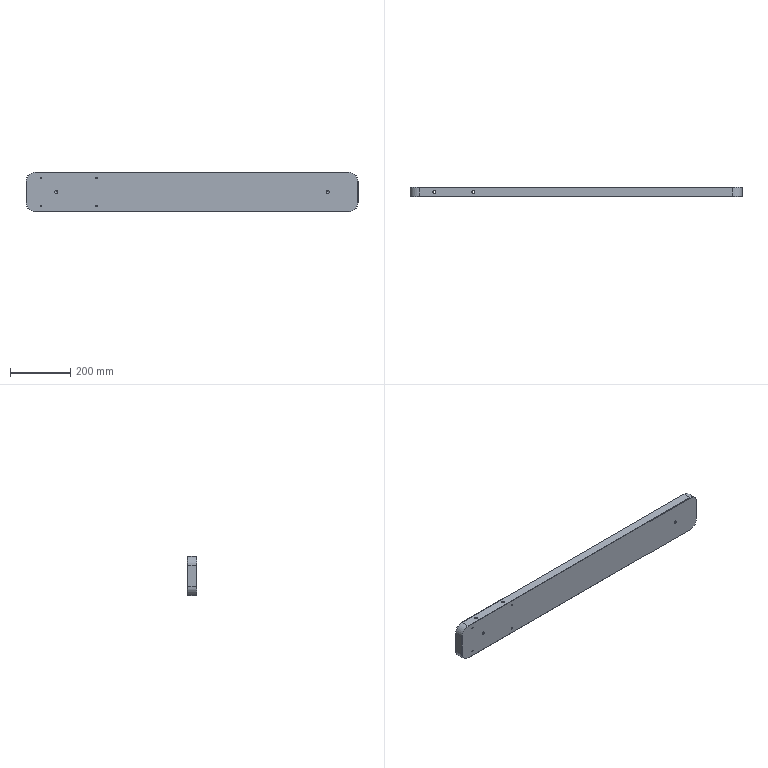Part | SolidWorks | features HoleWzd 3, Chamfer 1, Extrusion 1, Fillet 1 | 1 solid | 50 faces | box 1100 x 30 x 130 mm | volume 4243037 mm3 | cylinder 20 | cone 16 | plane 14 | commonest cylinder face diameters 5 x8 8.5 x4 10.2 x4 60 x4
STEP:
#1=CARTESIAN_POINT('',(-474.25,15.,64.225));
#2=VERTEX_POINT('',#1);
#3=CARTESIAN_POINT('',(-465.75,15.,64.225));
#4=VERTEX_POINT('',#3);
#5=CARTESIAN_POINT('',(-470.,15.,64.225));
#6=DIRECTION('',(0.,0.,1.));
#7=DIRECTION('',(1.,0.,0.));
#8=AXIS2_PLACEMENT_3D('',#5,#6,#7);
#9=CIRCLE('',#8,4.25);
#10=EDGE_CURVE('',#2,#4,#9,.T.);
#11=ORIENTED_EDGE('',*,*,#10,.F.);
#12=CARTESIAN_POINT('',(-475.025,15.,65.));
#13=VERTEX_POINT('',#12);
#14=CARTESIAN_POINT('',(-475.025,15.,65.));
#15=DIRECTION('',(-0.7071,0.,0.7071));
#16=VECTOR('',#15,1000.);
#17=LINE('',#14,#16);
#18=EDGE_CURVE('',#2,#13,#17,.T.);
#19=ORIENTED_EDGE('',*,*,#18,.T.);
#20=CARTESIAN_POINT('',(-464.975,15.,65.));
#21=VERTEX_POINT('',#20);
#22=CARTESIAN_POINT('',(-470.,15.,65.));
#23=DIRECTION('',(0.,0.,1.));
#24=DIRECTION('',(1.,0.,0.));
#25=AXIS2_PLACEMENT_3D('',#22,#23,#24);
#26=CIRCLE('',#25,5.025);
#27=EDGE_CURVE('',#13,#21,#26,.T.);
#28=ORIENTED_EDGE('',*,*,#27,.T.);
#29=CARTESIAN_POINT('',(-464.975,15.,65.));
#30=DIRECTION('',(0.7071,0.,0.7071));
#31=VECTOR('',#30,1000.);
#32=LINE('',#29,#31);
#33=EDGE_CURVE('',#4,#21,#32,.T.);
#34=ORIENTED_EDGE('',*,*,#33,.F.);
#35=EDGE_LOOP('',(#11,#19,#28,#34));
#36=FACE_OUTER_BOUND('',#35,.T.);
#37=CARTESIAN_POINT('',(-470.,15.,65.));
#38=DIRECTION('',(0.,0.,1.));
#39=DIRECTION('',(1.,0.,0.));
#40=AXIS2_PLACEMENT_3D('',#37,#38,#39);
#41=CONICAL_SURFACE('',#40,5.025,0.7854);
#42=ADVANCED_FACE('',(#36),#41,.F.);
#43=CARTESIAN_POINT('',(-474.25,15.,-65.));
#44=VERTEX_POINT('',#43);
#45=CARTESIAN_POINT('',(-465.75,15.,-65.));
#46=VERTEX_POINT('',#45);
#47=CARTESIAN_POINT('',(-470.,15.,-65.));
#48=DIRECTION('',(0.,0.,1.));
#49=DIRECTION('',(1.,0.,0.));
#50=AXIS2_PLACEMENT_3D('',#47,#48,#49);
#51=CIRCLE('',#50,4.25);
#52=EDGE_CURVE('',#44,#46,#51,.T.);
#53=ORIENTED_EDGE('',*,*,#52,.F.);
#54=CARTESIAN_POINT('',(-474.25,15.,65.));
#55=DIRECTION('',(0.,0.,1.));
#56=VECTOR('',#55,1000.);
#57=LINE('',#54,#56);
#58=EDGE_CURVE('',#44,#2,#57,.T.);
#59=ORIENTED_EDGE('',*,*,#58,.T.);
#60=ORIENTED_EDGE('',*,*,#10,.T.);
#61=CARTESIAN_POINT('',(-465.75,15.,65.));
#62=DIRECTION('',(0.,0.,1.));
#63=VECTOR('',#62,1000.);
#64=LINE('',#61,#63);
#65=EDGE_CURVE('',#46,#4,#64,.T.);
#66=ORIENTED_EDGE('',*,*,#65,.F.);
#67=EDGE_LOOP('',(#53,#59,#60,#66));
#68=FACE_OUTER_BOUND('',#67,.T.);
#69=CARTESIAN_POINT('',(-470.,15.,65.));
#70=DIRECTION('',(0.,0.,1.));
#71=DIRECTION('',(1.,0.,0.));
#72=AXIS2_PLACEMENT_3D('',#69,#70,#71);
#73=CYLINDRICAL_SURFACE('',#72,4.25);
#74=ADVANCED_FACE('',(#68),#73,.F.);
#75=CARTESIAN_POINT('',(-344.25,15.,64.225));
#76=VERTEX_POINT('',#75);
#77=CARTESIAN_POINT('',(-335.75,15.,64.225));
#78=VERTEX_POINT('',#77);
#79=CARTESIAN_POINT('',(-340.,15.,64.225));
#80=DIRECTION('',(0.,0.,1.));
#81=DIRECTION('',(1.,0.,0.));
#82=AXIS2_PLACEMENT_3D('',#79,#80,#81);
#83=CIRCLE('',#82,4.25);
#84=EDGE_CURVE('',#76,#78,#83,.T.);
#85=ORIENTED_EDGE('',*,*,#84,.F.);
#86=CARTESIAN_POINT('',(-345.025,15.,65.));
#87=VERTEX_POINT('',#86);
#88=CARTESIAN_POINT('',(-345.025,15.,65.));
#89=DIRECTION('',(-0.7071,0.,0.7071));
#90=VECTOR('',#89,1000.);
#91=LINE('',#88,#90);
#92=EDGE_CURVE('',#76,#87,#91,.T.);
#93=ORIENTED_EDGE('',*,*,#92,.T.);
#94=CARTESIAN_POINT('',(-334.975,15.,65.));
#95=VERTEX_POINT('',#94);
#96=CARTESIAN_POINT('',(-340.,15.,65.));
#97=DIRECTION('',(0.,0.,1.));
#98=DIRECTION('',(1.,0.,0.));
#99=AXIS2_PLACEMENT_3D('',#96,#97,#98);
#100=CIRCLE('',#99,5.025);
#101=EDGE_CURVE('',#87,#95,#100,.T.);
#102=ORIENTED_EDGE('',*,*,#101,.T.);
#103=CARTESIAN_POINT('',(-334.975,15.,65.));
#104=DIRECTION('',(0.7071,0.,0.7071));
#105=VECTOR('',#104,1000.);
#106=LINE('',#103,#105);
#107=EDGE_CURVE('',#78,#95,#106,.T.);
#108=ORIENTED_EDGE('',*,*,#107,.F.);
#109=EDGE_LOOP('',(#85,#93,#102,#108));
#110=FACE_OUTER_BOUND('',#109,.T.);
#111=CARTESIAN_POINT('',(-340.,15.,65.));
#112=DIRECTION('',(0.,0.,1.));
#113=DIRECTION('',(1.,0.,0.));
#114=AXIS2_PLACEMENT_3D('',#111,#112,#113);
#115=CONICAL_SURFACE('',#114,5.025,0.7854);
#116=ADVANCED_FACE('',(#110),#115,.F.);
#117=CARTESIAN_POINT('',(-344.25,15.,-65.));
#118=VERTEX_POINT('',#117);
#119=CARTESIAN_POINT('',(-335.75,15.,-65.));
#120=VERTEX_POINT('',#119);
#121=CARTESIAN_POINT('',(-340.,15.,-65.));
#122=DIRECTION('',(0.,0.,1.));
#123=DIRECTION('',(1.,0.,0.));
#124=AXIS2_PLACEMENT_3D('',#121,#122,#123);
#125=CIRCLE('',#124,4.25);
#126=EDGE_CURVE('',#118,#120,#125,.T.);
#127=ORIENTED_EDGE('',*,*,#126,.F.);
#128=CARTESIAN_POINT('',(-344.25,15.,65.));
#129=DIRECTION('',(0.,0.,1.));
#130=VECTOR('',#129,1000.);
#131=LINE('',#128,#130);
#132=EDGE_CURVE('',#118,#76,#131,.T.);
#133=ORIENTED_EDGE('',*,*,#132,.T.);
#134=ORIENTED_EDGE('',*,*,#84,.T.);
#135=CARTESIAN_POINT('',(-335.75,15.,65.));
#136=DIRECTION('',(0.,0.,1.));
#137=VECTOR('',#136,1000.);
#138=LINE('',#135,#137);
#139=EDGE_CURVE('',#120,#78,#138,.T.);
#140=ORIENTED_EDGE('',*,*,#139,.F.);
#141=EDGE_LOOP('',(#127,#133,#134,#140));
#142=FACE_OUTER_BOUND('',#141,.T.);
#143=CARTESIAN_POINT('',(-340.,15.,65.));
#144=DIRECTION('',(0.,0.,1.));
#145=DIRECTION('',(1.,0.,0.));
#146=AXIS2_PLACEMENT_3D('',#143,#144,#145);
#147=CYLINDRICAL_SURFACE('',#146,4.25);
#148=ADVANCED_FACE('',(#142),#147,.F.);
#149=CARTESIAN_POINT('',(450.,25.,5.1));
#150=VERTEX_POINT('',#149);
#151=CARTESIAN_POINT('',(450.,25.,-5.1));
#152=VERTEX_POINT('',#151);
#153=CARTESIAN_POINT('',(450.,25.,0.));
#154=DIRECTION('',(0.,-1.,0.));
#155=DIRECTION('',(0.,0.,-1.));
#156=AXIS2_PLACEMENT_3D('',#153,#154,#155);
#157=CIRCLE('',#156,5.1);
#158=EDGE_CURVE('',#150,#152,#157,.T.);
#159=ORIENTED_EDGE('',*,*,#158,.F.);
#160=CARTESIAN_POINT('',(450.,0.,5.1));
#161=VERTEX_POINT('',#160);
#162=CARTESIAN_POINT('',(450.,0.,5.1));
#163=DIRECTION('',(0.,-1.,0.));
#164=VECTOR('',#163,1000.);
#165=LINE('',#162,#164);
#166=EDGE_CURVE('',#150,#161,#165,.T.);
#167=ORIENTED_EDGE('',*,*,#166,.T.);
#168=CARTESIAN_POINT('',(450.,0.,-5.1));
#169=VERTEX_POINT('',#168);
#170=CARTESIAN_POINT('',(450.,0.,0.));
#171=DIRECTION('',(0.,-1.,0.));
#172=DIRECTION('',(0.,0.,-1.));
#173=AXIS2_PLACEMENT_3D('',#170,#171,#172);
#174=CIRCLE('',#173,5.1);
#175=EDGE_CURVE('',#161,#169,#174,.T.);
#176=ORIENTED_EDGE('',*,*,#175,.T.);
#177=CARTESIAN_POINT('',(450.,0.,-5.1));
#178=DIRECTION('',(0.,-1.,0.));
#179=VECTOR('',#178,1000.);
#180=LINE('',#177,#179);
#181=EDGE_CURVE('',#152,#169,#180,.T.);
#182=ORIENTED_EDGE('',*,*,#181,.F.);
#183=EDGE_LOOP('',(#159,#167,#176,#182));
#184=FACE_OUTER_BOUND('',#183,.T.);
#185=CARTESIAN_POINT('',(450.,0.,0.));
#186=DIRECTION('',(0.,-1.,0.));
#187=DIRECTION('',(0.,0.,-1.));
#188=AXIS2_PLACEMENT_3D('',#185,#186,#187);
#189=CYLINDRICAL_SURFACE('',#188,5.1);
#190=ADVANCED_FACE('',(#184),#189,.F.);
#191=CARTESIAN_POINT('',(450.,28.064,0.));
#192=VERTEX_POINT('',#191);
#193=CARTESIAN_POINT('',(450.,25.,-5.1));
#194=DIRECTION('',(0.,-0.515,-0.8572));
#195=VECTOR('',#194,1000.);
#196=LINE('',#193,#195);
#197=EDGE_CURVE('',#192,#152,#196,.T.);
#198=ORIENTED_EDGE('',*,*,#197,.F.);
#199=CARTESIAN_POINT('',(450.,25.,5.1));
#200=DIRECTION('',(0.,-0.515,0.8572));
#201=VECTOR('',#200,1000.);
#202=LINE('',#199,#201);
#203=EDGE_CURVE('',#192,#150,#202,.T.);
#204=ORIENTED_EDGE('',*,*,#203,.T.);
#205=ORIENTED_EDGE('',*,*,#158,.T.);
#206=EDGE_LOOP('',(#198,#204,#205));
#207=FACE_OUTER_BOUND('',#206,.T.);
#208=CARTESIAN_POINT('',(450.,25.,0.));
#209=DIRECTION('',(0.,-1.,0.));
#210=DIRECTION('',(0.,0.,-1.));
#211=AXIS2_PLACEMENT_3D('',#208,#209,#210);
#212=CONICAL_SURFACE('',#211,5.1,1.03);
#213=ADVANCED_FACE('',(#207),#212,.F.);
#214=CARTESIAN_POINT('',(-450.,25.,5.1));
#215=VERTEX_POINT('',#214);
#216=CARTESIAN_POINT('',(-450.,25.,-5.1));
#217=VERTEX_POINT('',#216);
#218=CARTESIAN_POINT('',(-450.,25.,0.));
#219=DIRECTION('',(0.,-1.,0.));
#220=DIRECTION('',(0.,0.,-1.));
#221=AXIS2_PLACEMENT_3D('',#218,#219,#220);
#222=CIRCLE('',#221,5.1);
#223=EDGE_CURVE('',#215,#217,#222,.T.);
#224=ORIENTED_EDGE('',*,*,#223,.F.);
#225=CARTESIAN_POINT('',(-450.,0.,5.1));
#226=VERTEX_POINT('',#225);
#227=CARTESIAN_POINT('',(-450.,0.,5.1));
#228=DIRECTION('',(0.,-1.,0.));
#229=VECTOR('',#228,1000.);
#230=LINE('',#227,#229);
#231=EDGE_CURVE('',#215,#226,#230,.T.);
#232=ORIENTED_EDGE('',*,*,#231,.T.);
#233=CARTESIAN_POINT('',(-450.,0.,-5.1));
#234=VERTEX_POINT('',#233);
#235=CARTESIAN_POINT('',(-450.,0.,0.));
#236=DIRECTION('',(0.,-1.,0.));
#237=DIRECTION('',(0.,0.,-1.));
#238=AXIS2_PLACEMENT_3D('',#235,#236,#237);
#239=CIRCLE('',#238,5.1);
#240=EDGE_CURVE('',#226,#234,#239,.T.);
#241=ORIENTED_EDGE('',*,*,#240,.T.);
#242=CARTESIAN_POINT('',(-450.,0.,-5.1));
#243=DIRECTION('',(0.,-1.,0.));
#244=VECTOR('',#243,1000.);
#245=LINE('',#242,#244);
#246=EDGE_CURVE('',#217,#234,#245,.T.);
#247=ORIENTED_EDGE('',*,*,#246,.F.);
#248=EDGE_LOOP('',(#224,#232,#241,#247));
#249=FACE_OUTER_BOUND('',#248,.T.);
#250=CARTESIAN_POINT('',(-450.,0.,0.));
#251=DIRECTION('',(0.,-1.,0.));
#252=DIRECTION('',(0.,0.,-1.));
#253=AXIS2_PLACEMENT_3D('',#250,#251,#252);
#254=CYLINDRICAL_SURFACE('',#253,5.1);
#255=ADVANCED_FACE('',(#249),#254,.F.);
#256=CARTESIAN_POINT('',(-450.,28.064,0.));
#257=VERTEX_POINT('',#256);
#258=CARTESIAN_POINT('',(-450.,25.,-5.1));
#259=DIRECTION('',(0.,-0.515,-0.8572));
#260=VECTOR('',#259,1000.);
#261=LINE('',#258,#260);
#262=EDGE_CURVE('',#257,#217,#261,.T.);
#263=ORIENTED_EDGE('',*,*,#262,.F.);
#264=CARTESIAN_POINT('',(-450.,25.,5.1));
#265=DIRECTION('',(0.,-0.515,0.8572));
#266=VECTOR('',#265,1000.);
#267=LINE('',#264,#266);
#268=EDGE_CURVE('',#257,#215,#267,.T.);
#269=ORIENTED_EDGE('',*,*,#268,.T.);
#270=ORIENTED_EDGE('',*,*,#223,.T.);
#271=EDGE_LOOP('',(#263,#269,#270));
#272=FACE_OUTER_BOUND('',#271,.T.);
#273=CARTESIAN_POINT('',(-450.,25.,0.));
#274=DIRECTION('',(0.,-1.,0.));
#275=DIRECTION('',(0.,0.,-1.));
#276=AXIS2_PLACEMENT_3D('',#273,#274,#275);
#277=CONICAL_SURFACE('',#276,5.1,1.03);
#278=ADVANCED_FACE('',(#272),#277,.F.);
#279=CARTESIAN_POINT('',(-316.,0.,-49.5));
#280=VERTEX_POINT('',#279);
#281=CARTESIAN_POINT('',(-316.,0.,-44.5));
#282=VERTEX_POINT('',#281);
#283=CARTESIAN_POINT('',(-316.,0.,-47.));
#284=DIRECTION('',(0.,1.,0.));
#285=DIRECTION('',(0.,0.,1.));
#286=AXIS2_PLACEMENT_3D('',#283,#284,#285);
#287=CIRCLE('',#286,2.5);
#288=EDGE_CURVE('',#280,#282,#287,.T.);
#289=ORIENTED_EDGE('',*,*,#288,.F.);
#290=CARTESIAN_POINT('',(-316.,30.,-49.5));
#291=VERTEX_POINT('',#290);
#292=CARTESIAN_POINT('',(-316.,30.,-49.5));
#293=DIRECTION('',(0.,1.,0.));
#294=VECTOR('',#293,1000.);
#295=LINE('',#292,#294);
#296=EDGE_CURVE('',#280,#291,#295,.T.);
#297=ORIENTED_EDGE('',*,*,#296,.T.);
#298=CARTESIAN_POINT('',(-316.,30.,-44.5));
#299=VERTEX_POINT('',#298);
#300=CARTESIAN_POINT('',(-316.,30.,-47.));
#301=DIRECTION('',(0.,1.,0.));
#302=DIRECTION('',(0.,0.,1.));
#303=AXIS2_PLACEMENT_3D('',#300,#301,#302);
#304=CIRCLE('',#303,2.5);
#305=EDGE_CURVE('',#291,#299,#304,.T.);
#306=ORIENTED_EDGE('',*,*,#305,.T.);
#307=CARTESIAN_POINT('',(-316.,30.,-44.5));
#308=DIRECTION('',(0.,1.,0.));
#309=VECTOR('',#308,1000.);
#310=LINE('',#307,#309);
#311=EDGE_CURVE('',#282,#299,#310,.T.);
#312=ORIENTED_EDGE('',*,*,#311,.F.);
#313=EDGE_LOOP('',(#289,#297,#306,#312));
#314=FACE_OUTER_BOUND('',#313,.T.);
#315=CARTESIAN_POINT('',(-316.,30.,-47.));
#316=DIRECTION('',(0.,1.,0.));
#317=DIRECTION('',(0.,0.,1.));
#318=AXIS2_PLACEMENT_3D('',#315,#316,#317);
#319=CYLINDRICAL_SURFACE('',#318,2.5);
#320=ADVANCED_FACE('',(#314),#319,.F.);
#321=CARTESIAN_POINT('',(-316.,0.,44.5));
#322=VERTEX_POINT('',#321);
#323=CARTESIAN_POINT('',(-316.,0.,49.5));
#324=VERTEX_POINT('',#323);
#325=CARTESIAN_POINT('',(-316.,0.,47.));
#326=DIRECTION('',(0.,1.,0.));
#327=DIRECTION('',(0.,0.,1.));
#328=AXIS2_PLACEMENT_3D('',#325,#326,#327);
#329=CIRCLE('',#328,2.5);
#330=EDGE_CURVE('',#322,#324,#329,.T.);
#331=ORIENTED_EDGE('',*,*,#330,.F.);
#332=CARTESIAN_POINT('',(-316.,30.,44.5));
#333=VERTEX_POINT('',#332);
#334=CARTESIAN_POINT('',(-316.,30.,44.5));
#335=DIRECTION('',(0.,1.,0.));
#336=VECTOR('',#335,1000.);
#337=LINE('',#334,#336);
#338=EDGE_CURVE('',#322,#333,#337,.T.);
#339=ORIENTED_EDGE('',*,*,#338,.T.);
#340=CARTESIAN_POINT('',(-316.,30.,49.5));
#341=VERTEX_POINT('',#340);
#342=CARTESIAN_POINT('',(-316.,30.,47.));
#343=DIRECTION('',(0.,1.,0.));
#344=DIRECTION('',(0.,0.,1.));
#345=AXIS2_PLACEMENT_3D('',#342,#343,#344);
#346=CIRCLE('',#345,2.5);
#347=EDGE_CURVE('',#333,#341,#346,.T.);
#348=ORIENTED_EDGE('',*,*,#347,.T.);
#349=CARTESIAN_POINT('',(-316.,30.,49.5));
#350=DIRECTION('',(0.,1.,0.));
#351=VECTOR('',#350,1000.);
#352=LINE('',#349,#351);
#353=EDGE_CURVE('',#324,#341,#352,.T.);
#354=ORIENTED_EDGE('',*,*,#353,.F.);
#355=EDGE_LOOP('',(#331,#339,#348,#354));
#356=FACE_OUTER_BOUND('',#355,.T.);
#357=CARTESIAN_POINT('',(-316.,30.,47.));
#358=DIRECTION('',(0.,1.,0.));
#359=DIRECTION('',(0.,0.,1.));
#360=AXIS2_PLACEMENT_3D('',#357,#358,#359);
#361=CYLINDRICAL_SURFACE('',#360,2.5);
#362=ADVANCED_FACE('',(#356),#361,.F.);
#363=CARTESIAN_POINT('',(-500.,0.,-49.5));
#364=VERTEX_POINT('',#363);
#365=CARTESIAN_POINT('',(-500.,0.,-44.5));
#366=VERTEX_POINT('',#365);
#367=CARTESIAN_POINT('',(-500.,0.,-47.));
#368=DIRECTION('',(0.,1.,0.));
#369=DIRECTION('',(0.,0.,1.));
#370=AXIS2_PLACEMENT_3D('',#367,#368,#369);
#371=CIRCLE('',#370,2.5);
#372=EDGE_CURVE('',#364,#366,#371,.T.);
#373=ORIENTED_EDGE('',*,*,#372,.F.);
#374=CARTESIAN_POINT('',(-500.,30.,-49.5));
#375=VERTEX_POINT('',#374);
#376=CARTESIAN_POINT('',(-500.,30.,-49.5));
#377=DIRECTION('',(0.,1.,0.));
#378=VECTOR('',#377,1000.);
#379=LINE('',#376,#378);
#380=EDGE_CURVE('',#364,#375,#379,.T.);
#381=ORIENTED_EDGE('',*,*,#380,.T.);
#382=CARTESIAN_POINT('',(-500.,30.,-44.5));
#383=VERTEX_POINT('',#382);
#384=CARTESIAN_POINT('',(-500.,30.,-47.));
#385=DIRECTION('',(0.,1.,0.));
#386=DIRECTION('',(0.,0.,1.));
#387=AXIS2_PLACEMENT_3D('',#384,#385,#386);
#388=CIRCLE('',#387,2.5);
#389=EDGE_CURVE('',#375,#383,#388,.T.);
#390=ORIENTED_EDGE('',*,*,#389,.T.);
#391=CARTESIAN_POINT('',(-500.,30.,-44.5));
#392=DIRECTION('',(0.,1.,0.));
#393=VECTOR('',#392,1000.);
#394=LINE('',#391,#393);
#395=EDGE_CURVE('',#366,#383,#394,.T.);
#396=ORIENTED_EDGE('',*,*,#395,.F.);
#397=EDGE_LOOP('',(#373,#381,#390,#396));
#398=FACE_OUTER_BOUND('',#397,.T.);
#399=CARTESIAN_POINT('',(-500.,30.,-47.));
#400=DIRECTION('',(0.,1.,0.));
#401=DIRECTION('',(0.,0.,1.));
#402=AXIS2_PLACEMENT_3D('',#399,#400,#401);
#403=CYLINDRICAL_SURFACE('',#402,2.5);
#404=ADVANCED_FACE('',(#398),#403,.F.);
#405=CARTESIAN_POINT('',(-500.,0.,44.5));
#406=VERTEX_POINT('',#405);
#407=CARTESIAN_POINT('',(-500.,0.,49.5));
#408=VERTEX_POINT('',#407);
#409=CARTESIAN_POINT('',(-500.,0.,47.));
#410=DIRECTION('',(0.,1.,0.));
#411=DIRECTION('',(0.,0.,1.));
#412=AXIS2_PLACEMENT_3D('',#409,#410,#411);
#413=CIRCLE('',#412,2.5);
#414=EDGE_CURVE('',#406,#408,#413,.T.);
#415=ORIENTED_EDGE('',*,*,#414,.F.);
#416=CARTESIAN_POINT('',(-500.,30.,44.5));
#417=VERTEX_POINT('',#416);
#418=CARTESIAN_POINT('',(-500.,30.,44.5));
#419=DIRECTION('',(0.,1.,0.));
#420=VECTOR('',#419,1000.);
#421=LINE('',#418,#420);
#422=EDGE_CURVE('',#406,#417,#421,.T.);
#423=ORIENTED_EDGE('',*,*,#422,.T.);
#424=CARTESIAN_POINT('',(-500.,30.,49.5));
#425=VERTEX_POINT('',#424);
#426=CARTESIAN_POINT('',(-500.,30.,47.));
#427=DIRECTION('',(0.,1.,0.));
#428=DIRECTION('',(0.,0.,1.));
#429=AXIS2_PLACEMENT_3D('',#426,#427,#428);
#430=CIRCLE('',#429,2.5);
#431=EDGE_CURVE('',#417,#425,#430,.T.);
#432=ORIENTED_EDGE('',*,*,#431,.T.);
#433=CARTESIAN_POINT('',(-500.,30.,49.5));
#434=DIRECTION('',(0.,1.,0.));
#435=VECTOR('',#434,1000.);
#436=LINE('',#433,#435);
#437=EDGE_CURVE('',#408,#425,#436,.T.);
#438=ORIENTED_EDGE('',*,*,#437,.F.);
#439=EDGE_LOOP('',(#415,#423,#432,#438));
#440=FACE_OUTER_BOUND('',#439,.T.);
#441=CARTESIAN_POINT('',(-500.,30.,47.));
#442=DIRECTION('',(0.,1.,0.));
#443=DIRECTION('',(0.,0.,1.));
#444=AXIS2_PLACEMENT_3D('',#441,#442,#443);
#445=CYLINDRICAL_SURFACE('',#444,2.5);
#446=ADVANCED_FACE('',(#440),#445,.F.);
#447=CARTESIAN_POINT('',(550.,29.,35.));
#448=VERTEX_POINT('',#447);
#449=CARTESIAN_POINT('',(550.,1.,35.));
#450=VERTEX_POINT('',#449);
#451=CARTESIAN_POINT('',(550.,30.,35.));
#452=DIRECTION('',(0.,-1.,0.));
#453=VECTOR('',#452,1000.);
#454=LINE('',#451,#453);
#455=EDGE_CURVE('',#448,#450,#454,.T.);
#456=ORIENTED_EDGE('',*,*,#455,.T.);
#457=CARTESIAN_POINT('',(550.,1.,-35.));
#458=VERTEX_POINT('',#457);
#459=CARTESIAN_POINT('',(550.,1.,-35.));
#460=DIRECTION('',(0.,0.,-1.));
#461=VECTOR('',#460,1000.);
#462=LINE('',#459,#461);
#463=EDGE_CURVE('',#450,#458,#462,.T.);
#464=ORIENTED_EDGE('',*,*,#463,.T.);
#465=CARTESIAN_POINT('',(550.,29.,-35.));
#466=VERTEX_POINT('',#465);
#467=CARTESIAN_POINT('',(550.,30.,-35.));
#468=DIRECTION('',(0.,1.,0.));
#469=VECTOR('',#468,1000.);
#470=LINE('',#467,#469);
#471=EDGE_CURVE('',#458,#466,#470,.T.);
#472=ORIENTED_EDGE('',*,*,#471,.T.);
#473=CARTESIAN_POINT('',(550.,29.,65.));
#474=DIRECTION('',(0.,0.,1.));
#475=VECTOR('',#474,1000.);
#476=LINE('',#473,#475);
#477=EDGE_CURVE('',#466,#448,#476,.T.);
#478=ORIENTED_EDGE('',*,*,#477,.T.);
#479=EDGE_LOOP('',(#456,#464,#472,#478));
#480=FACE_OUTER_BOUND('',#479,.T.);
#481=CARTESIAN_POINT('',(550.,30.,65.));
#482=DIRECTION('',(-1.,0.,0.));
#483=DIRECTION('',(0.,0.,1.));
#484=AXIS2_PLACEMENT_3D('',#481,#482,#483);
#485=PLANE('',#484);
#486=ADVANCED_FACE('',(#480),#485,.F.);
#487=CARTESIAN_POINT('',(-470.,15.,-65.));
#488=DIRECTION('',(0.,0.,1.));
#489=DIRECTION('',(1.,0.,0.));
#490=AXIS2_PLACEMENT_3D('',#487,#488,#489);
#491=CIRCLE('',#490,4.25);
#492=EDGE_CURVE('',#46,#44,#491,.T.);
#493=ORIENTED_EDGE('',*,*,#492,.T.);
#494=ORIENTED_EDGE('',*,*,#52,.T.);
#495=EDGE_LOOP('',(#493,#494));
#496=FACE_BOUND('',#495,.T.);
#497=CARTESIAN_POINT('',(-340.,15.,-65.));
#498=DIRECTION('',(0.,0.,1.));
#499=DIRECTION('',(1.,0.,0.));
#500=AXIS2_PLACEMENT_3D('',#497,#498,#499);
#501=CIRCLE('',#500,4.25);
#502=EDGE_CURVE('',#120,#118,#501,.T.);
#503=ORIENTED_EDGE('',*,*,#502,.T.);
#504=ORIENTED_EDGE('',*,*,#126,.T.);
#505=EDGE_LOOP('',(#503,#504));
#506=FACE_BOUND('',#505,.T.);
#507=CARTESIAN_POINT('',(520.,29.,-65.));
#508=VERTEX_POINT('',#507);
#509=CARTESIAN_POINT('',(520.,1.,-65.));
#510=VERTEX_POINT('',#509);
#511=CARTESIAN_POINT('',(520.,30.,-65.));
#512=DIRECTION('',(0.,-1.,0.));
#513=VECTOR('',#512,1000.);
#514=LINE('',#511,#513);
#515=EDGE_CURVE('',#508,#510,#514,.T.);
#516=ORIENTED_EDGE('',*,*,#515,.T.);
#517=CARTESIAN_POINT('',(-520.,1.,-65.));
#518=VERTEX_POINT('',#517);
#519=CARTESIAN_POINT('',(-520.,1.,-65.));
#520=DIRECTION('',(-1.,0.,0.));
#521=VECTOR('',#520,1000.);
#522=LINE('',#519,#521);
#523=EDGE_CURVE('',#510,#518,#522,.T.);
#524=ORIENTED_EDGE('',*,*,#523,.T.);
#525=CARTESIAN_POINT('',(-520.,29.,-65.));
#526=VERTEX_POINT('',#525);
#527=CARTESIAN_POINT('',(-520.,30.,-65.));
#528=DIRECTION('',(0.,1.,0.));
#529=VECTOR('',#528,1000.);
#530=LINE('',#527,#529);
#531=EDGE_CURVE('',#518,#526,#530,.T.);
#532=ORIENTED_EDGE('',*,*,#531,.T.);
#533=CARTESIAN_POINT('',(-550.,29.,-65.));
#534=DIRECTION('',(1.,0.,0.));
#535=VECTOR('',#534,1000.);
#536=LINE('',#533,#535);
#537=EDGE_CURVE('',#526,#508,#536,.T.);
#538=ORIENTED_EDGE('',*,*,#537,.T.);
#539=EDGE_LOOP('',(#516,#524,#532,#538));
#540=FACE_OUTER_BOUND('',#539,.T.);
#541=CARTESIAN_POINT('',(-550.,30.,-65.));
#542=DIRECTION('',(0.,0.,1.));
#543=DIRECTION('',(1.,0.,0.));
#544=AXIS2_PLACEMENT_3D('',#541,#542,#543);
#545=PLANE('',#544);
#546=ADVANCED_FACE('',(#496,#506,#540),#545,.F.);
#547=CARTESIAN_POINT('',(-550.,29.,-35.));
#548=VERTEX_POINT('',#547);
#549=CARTESIAN_POINT('',(-550.,1.,-35.));
#550=VERTEX_POINT('',#549);
#551=CARTESIAN_POINT('',(-550.,30.,-35.));
#552=DIRECTION('',(0.,-1.,0.));
#553=VECTOR('',#552,1000.);
#554=LINE('',#551,#553);
#555=EDGE_CURVE('',#548,#550,#554,.T.);
#556=ORIENTED_EDGE('',*,*,#555,.T.);
#557=CARTESIAN_POINT('',(-550.,1.,35.));
#558=VERTEX_POINT('',#557);
#559=CARTESIAN_POINT('',(-550.,1.,35.));
#560=DIRECTION('',(0.,0.,1.));
#561=VECTOR('',#560,1000.);
#562=LINE('',#559,#561);
#563=EDGE_CURVE('',#550,#558,#562,.T.);
#564=ORIENTED_EDGE('',*,*,#563,.T.);
#565=CARTESIAN_POINT('',(-550.,29.,35.));
#566=VERTEX_POINT('',#565);
#567=CARTESIAN_POINT('',(-550.,30.,35.));
#568=DIRECTION('',(0.,1.,0.));
#569=VECTOR('',#568,1000.);
#570=LINE('',#567,#569);
#571=EDGE_CURVE('',#558,#566,#570,.T.);
#572=ORIENTED_EDGE('',*,*,#571,.T.);
#573=CARTESIAN_POINT('',(-550.,29.,65.));
#574=DIRECTION('',(0.,0.,-1.));
#575=VECTOR('',#574,1000.);
#576=LINE('',#573,#575);
#577=EDGE_CURVE('',#566,#548,#576,.T.);
#578=ORIENTED_EDGE('',*,*,#577,.T.);
#579=EDGE_LOOP('',(#556,#564,#572,#578));
#580=FACE_OUTER_BOUND('',#579,.T.);
#581=CARTESIAN_POINT('',(-550.,30.,65.));
#582=DIRECTION('',(1.,0.,0.));
#583=DIRECTION('',(0.,0.,-1.));
#584=AXIS2_PLACEMENT_3D('',#581,#582,#583);
#585=PLANE('',#584);
#586=ADVANCED_FACE('',(#580),#585,.F.);
#587=CARTESIAN_POINT('',(-470.,15.,65.));
#588=DIRECTION('',(0.,0.,1.));
#589=DIRECTION('',(1.,0.,0.));
#590=AXIS2_PLACEMENT_3D('',#587,#588,#589);
#591=CIRCLE('',#590,5.025);
#592=EDGE_CURVE('',#21,#13,#591,.T.);
#593=ORIENTED_EDGE('',*,*,#592,.F.);
#594=ORIENTED_EDGE('',*,*,#27,.F.);
#595=EDGE_LOOP('',(#593,#594));
#596=FACE_BOUND('',#595,.T.);
#597=CARTESIAN_POINT('',(-340.,15.,65.));
#598=DIRECTION('',(0.,0.,1.));
#599=DIRECTION('',(1.,0.,0.));
#600=AXIS2_PLACEMENT_3D('',#597,#598,#599);
#601=CIRCLE('',#600,5.025);
#602=EDGE_CURVE('',#95,#87,#601,.T.);
#603=ORIENTED_EDGE('',*,*,#602,.F.);
#604=ORIENTED_EDGE('',*,*,#101,.F.);
#605=EDGE_LOOP('',(#603,#604));
#606=FACE_BOUND('',#605,.T.);
#607=CARTESIAN_POINT('',(-520.,29.,65.));
#608=VERTEX_POINT('',#607);
#609=CARTESIAN_POINT('',(-520.,1.,65.));
#610=VERTEX_POINT('',#609);
#611=CARTESIAN_POINT('',(-520.,30.,65.));
#612=DIRECTION('',(0.,-1.,0.));
#613=VECTOR('',#612,1000.);
#614=LINE('',#611,#613);
#615=EDGE_CURVE('',#608,#610,#614,.T.);
#616=ORIENTED_EDGE('',*,*,#615,.T.);
#617=CARTESIAN_POINT('',(520.,1.,65.));
#618=VERTEX_POINT('',#617);
#619=CARTESIAN_POINT('',(520.,1.,65.));
#620=DIRECTION('',(1.,0.,0.));
#621=VECTOR('',#620,1000.);
#622=LINE('',#619,#621);
#623=EDGE_CURVE('',#610,#618,#622,.T.);
#624=ORIENTED_EDGE('',*,*,#623,.T.);
#625=CARTESIAN_POINT('',(520.,29.,65.));
#626=VERTEX_POINT('',#625);
#627=CARTESIAN_POINT('',(520.,30.,65.));
#628=DIRECTION('',(0.,1.,0.));
#629=VECTOR('',#628,1000.);
#630=LINE('',#627,#629);
#631=EDGE_CURVE('',#618,#626,#630,.T.);
#632=ORIENTED_EDGE('',*,*,#631,.T.);
#633=CARTESIAN_POINT('',(-550.,29.,65.));
#634=DIRECTION('',(-1.,0.,0.));
#635=VECTOR('',#634,1000.);
#636=LINE('',#633,#635);
#637=EDGE_CURVE('',#626,#608,#636,.T.);
#638=ORIENTED_EDGE('',*,*,#637,.T.);
#639=EDGE_LOOP('',(#616,#624,#632,#638));
#640=FACE_OUTER_BOUND('',#639,.T.);
#641=CARTESIAN_POINT('',(-550.,30.,65.));
#642=DIRECTION('',(0.,0.,-1.));
#643=DIRECTION('',(-1.,0.,0.));
#644=AXIS2_PLACEMENT_3D('',#641,#642,#643);
#645=PLANE('',#644);
#646=ADVANCED_FACE('',(#596,#606,#640),#645,.F.);
#647=CARTESIAN_POINT('',(520.,30.,64.));
#648=VERTEX_POINT('',#647);
#649=CARTESIAN_POINT('',(549.,30.,35.));
#650=VERTEX_POINT('',#649);
#651=CARTESIAN_POINT('',(520.,30.,35.));
#652=DIRECTION('',(0.,1.,0.));
#653=DIRECTION('',(0.,0.,-1.));
#654=AXIS2_PLACEMENT_3D('',#651,#652,#653);
#655=CIRCLE('',#654,29.);
#656=EDGE_CURVE('',#648,#650,#655,.T.);
#657=ORIENTED_EDGE('',*,*,#656,.T.);
#658=CARTESIAN_POINT('',(549.,30.,-35.));
#659=VERTEX_POINT('',#658);
#660=CARTESIAN_POINT('',(549.,30.,0.));
#661=DIRECTION('',(0.,0.,-1.));
#662=VECTOR('',#661,1000.);
#663=LINE('',#660,#662);
#664=EDGE_CURVE('',#650,#659,#663,.T.);
#665=ORIENTED_EDGE('',*,*,#664,.T.);
#666=CARTESIAN_POINT('',(520.,30.,-64.));
#667=VERTEX_POINT('',#666);
#668=CARTESIAN_POINT('',(520.,30.,-35.));
#669=DIRECTION('',(0.,1.,0.));
#670=DIRECTION('',(0.,0.,-1.));
#671=AXIS2_PLACEMENT_3D('',#668,#669,#670);
#672=CIRCLE('',#671,29.);
#673=EDGE_CURVE('',#659,#667,#672,.T.);
#674=ORIENTED_EDGE('',*,*,#673,.T.);
#675=CARTESIAN_POINT('',(-520.,30.,-64.));
#676=VERTEX_POINT('',#675);
#677=CARTESIAN_POINT('',(0.,30.,-64.));
#678=DIRECTION('',(-1.,0.,0.));
#679=VECTOR('',#678,1000.);
#680=LINE('',#677,#679);
#681=EDGE_CURVE('',#667,#676,#680,.T.);
#682=ORIENTED_EDGE('',*,*,#681,.T.);
#683=CARTESIAN_POINT('',(-549.,30.,-35.));
#684=VERTEX_POINT('',#683);
#685=CARTESIAN_POINT('',(-520.,30.,-35.));
#686=DIRECTION('',(0.,1.,0.));
#687=DIRECTION('',(0.,0.,-1.));
#688=AXIS2_PLACEMENT_3D('',#685,#686,#687);
#689=CIRCLE('',#688,29.);
#690=EDGE_CURVE('',#676,#684,#689,.T.);
#691=ORIENTED_EDGE('',*,*,#690,.T.);
#692=CARTESIAN_POINT('',(-549.,30.,35.));
#693=VERTEX_POINT('',#692);
#694=CARTESIAN_POINT('',(-549.,30.,0.));
#695=DIRECTION('',(0.,0.,1.));
#696=VECTOR('',#695,1000.);
#697=LINE('',#694,#696);
#698=EDGE_CURVE('',#684,#693,#697,.T.);
#699=ORIENTED_EDGE('',*,*,#698,.T.);
#700=CARTESIAN_POINT('',(-520.,30.,64.));
#701=VERTEX_POINT('',#700);
#702=CARTESIAN_POINT('',(-520.,30.,35.));
#703=DIRECTION('',(0.,1.,0.));
#704=DIRECTION('',(0.,0.,-1.));
#705=AXIS2_PLACEMENT_3D('',#702,#703,#704);
#706=CIRCLE('',#705,29.);
#707=EDGE_CURVE('',#693,#701,#706,.T.);
#708=ORIENTED_EDGE('',*,*,#707,.T.);
#709=CARTESIAN_POINT('',(0.,30.,64.));
#710=DIRECTION('',(1.,0.,0.));
#711=VECTOR('',#710,1000.);
#712=LINE('',#709,#711);
#713=EDGE_CURVE('',#701,#648,#712,.T.);
#714=ORIENTED_EDGE('',*,*,#713,.T.);
#715=EDGE_LOOP('',(#657,#665,#674,#682,#691,#699,#708,#714));
#716=FACE_OUTER_BOUND('',#715,.T.);
#717=CARTESIAN_POINT('',(-316.,30.,-47.));
#718=DIRECTION('',(0.,1.,0.));
#719=DIRECTION('',(0.,0.,1.));
#720=AXIS2_PLACEMENT_3D('',#717,#718,#719);
#721=CIRCLE('',#720,2.5);
#722=EDGE_CURVE('',#299,#291,#721,.T.);
#723=ORIENTED_EDGE('',*,*,#722,.F.);
#724=ORIENTED_EDGE('',*,*,#305,.F.);
#725=EDGE_LOOP('',(#723,#724));
#726=FACE_BOUND('',#725,.T.);
#727=CARTESIAN_POINT('',(-316.,30.,47.));
#728=DIRECTION('',(0.,1.,0.));
#729=DIRECTION('',(0.,0.,1.));
#730=AXIS2_PLACEMENT_3D('',#727,#728,#729);
#731=CIRCLE('',#730,2.5);
#732=EDGE_CURVE('',#341,#333,#731,.T.);
#733=ORIENTED_EDGE('',*,*,#732,.F.);
#734=ORIENTED_EDGE('',*,*,#347,.F.);
#735=EDGE_LOOP('',(#733,#734));
#736=FACE_BOUND('',#735,.T.);
#737=CARTESIAN_POINT('',(-500.,30.,-47.));
#738=DIRECTION('',(0.,1.,0.));
#739=DIRECTION('',(0.,0.,1.));
#740=AXIS2_PLACEMENT_3D('',#737,#738,#739);
#741=CIRCLE('',#740,2.5);
#742=EDGE_CURVE('',#383,#375,#741,.T.);
#743=ORIENTED_EDGE('',*,*,#742,.F.);
#744=ORIENTED_EDGE('',*,*,#389,.F.);
#745=EDGE_LOOP('',(#743,#744));
#746=FACE_BOUND('',#745,.T.);
#747=CARTESIAN_POINT('',(-500.,30.,47.));
#748=DIRECTION('',(0.,1.,0.));
#749=DIRECTION('',(0.,0.,1.));
#750=AXIS2_PLACEMENT_3D('',#747,#748,#749);
#751=CIRCLE('',#750,2.5);
#752=EDGE_CURVE('',#425,#417,#751,.T.);
#753=ORIENTED_EDGE('',*,*,#752,.F.);
#754=ORIENTED_EDGE('',*,*,#431,.F.);
#755=EDGE_LOOP('',(#753,#754));
#756=FACE_BOUND('',#755,.T.);
#757=CARTESIAN_POINT('',(0.,30.,0.));
#758=DIRECTION('',(0.,-1.,0.));
#759=DIRECTION('',(0.,0.,-1.));
#760=AXIS2_PLACEMENT_3D('',#757,#758,#759);
#761=PLANE('',#760);
#762=ADVANCED_FACE('',(#716,#726,#736,#746,#756),#761,.F.);
#763=CARTESIAN_POINT('',(549.,0.,35.));
#764=VERTEX_POINT('',#763);
#765=CARTESIAN_POINT('',(520.,0.,64.));
#766=VERTEX_POINT('',#765);
#767=CARTESIAN_POINT('',(520.,0.,35.));
#768=DIRECTION('',(0.,-1.,0.));
#769=DIRECTION('',(0.,0.,-1.));
#770=AXIS2_PLACEMENT_3D('',#767,#768,#769);
#771=CIRCLE('',#770,29.);
#772=EDGE_CURVE('',#764,#766,#771,.T.);
#773=ORIENTED_EDGE('',*,*,#772,.T.);
#774=CARTESIAN_POINT('',(-520.,0.,64.));
#775=VERTEX_POINT('',#774);
#776=CARTESIAN_POINT('',(-520.,0.,64.));
#777=DIRECTION('',(-1.,0.,0.));
#778=VECTOR('',#777,1000.);
#779=LINE('',#776,#778);
#780=EDGE_CURVE('',#766,#775,#779,.T.);
#781=ORIENTED_EDGE('',*,*,#780,.T.);
#782=CARTESIAN_POINT('',(-549.,0.,35.));
#783=VERTEX_POINT('',#782);
#784=CARTESIAN_POINT('',(-520.,0.,35.));
#785=DIRECTION('',(0.,-1.,0.));
#786=DIRECTION('',(0.,0.,-1.));
#787=AXIS2_PLACEMENT_3D('',#784,#785,#786);
#788=CIRCLE('',#787,29.);
#789=EDGE_CURVE('',#775,#783,#788,.T.);
#790=ORIENTED_EDGE('',*,*,#789,.T.);
#791=CARTESIAN_POINT('',(-549.,0.,-35.));
#792=VERTEX_POINT('',#791);
#793=CARTESIAN_POINT('',(-549.,0.,-35.));
#794=DIRECTION('',(0.,0.,-1.));
#795=VECTOR('',#794,1000.);
#796=LINE('',#793,#795);
#797=EDGE_CURVE('',#783,#792,#796,.T.);
#798=ORIENTED_EDGE('',*,*,#797,.T.);
#799=CARTESIAN_POINT('',(-520.,0.,-64.));
#800=VERTEX_POINT('',#799);
#801=CARTESIAN_POINT('',(-520.,0.,-35.));
#802=DIRECTION('',(0.,-1.,0.));
#803=DIRECTION('',(0.,0.,-1.));
#804=AXIS2_PLACEMENT_3D('',#801,#802,#803);
#805=CIRCLE('',#804,29.);
#806=EDGE_CURVE('',#792,#800,#805,.T.);
#807=ORIENTED_EDGE('',*,*,#806,.T.);
#808=CARTESIAN_POINT('',(520.,0.,-64.));
#809=VERTEX_POINT('',#808);
#810=CARTESIAN_POINT('',(520.,0.,-64.));
#811=DIRECTION('',(1.,0.,0.));
#812=VECTOR('',#811,1000.);
#813=LINE('',#810,#812);
#814=EDGE_CURVE('',#800,#809,#813,.T.);
#815=ORIENTED_EDGE('',*,*,#814,.T.);
#816=CARTESIAN_POINT('',(549.,0.,-35.));
#817=VERTEX_POINT('',#816);
#818=CARTESIAN_POINT('',(520.,0.,-35.));
#819=DIRECTION('',(0.,-1.,0.));
#820=DIRECTION('',(0.,0.,-1.));
#821=AXIS2_PLACEMENT_3D('',#818,#819,#820);
#822=CIRCLE('',#821,29.);
#823=EDGE_CURVE('',#809,#817,#822,.T.);
#824=ORIENTED_EDGE('',*,*,#823,.T.);
#825=CARTESIAN_POINT('',(549.,0.,35.));
#826=DIRECTION('',(0.,0.,1.));
#827=VECTOR('',#826,1000.);
#828=LINE('',#825,#827);
#829=EDGE_CURVE('',#817,#764,#828,.T.);
#830=ORIENTED_EDGE('',*,*,#829,.T.);
#831=EDGE_LOOP('',(#773,#781,#790,#798,#807,#815,#824,#830));
#832=FACE_OUTER_BOUND('',#831,.T.);
#833=CARTESIAN_POINT('',(450.,0.,0.));
#834=DIRECTION('',(0.,-1.,0.));
#835=DIRECTION('',(0.,0.,-1.));
#836=AXIS2_PLACEMENT_3D('',#833,#834,#835);
#837=CIRCLE('',#836,5.1);
#838=EDGE_CURVE('',#169,#161,#837,.T.);
#839=ORIENTED_EDGE('',*,*,#838,.F.);
#840=ORIENTED_EDGE('',*,*,#175,.F.);
#841=EDGE_LOOP('',(#839,#840));
#842=FACE_BOUND('',#841,.T.);
#843=CARTESIAN_POINT('',(-450.,0.,0.));
#844=DIRECTION('',(0.,-1.,0.));
#845=DIRECTION('',(0.,0.,-1.));
#846=AXIS2_PLACEMENT_3D('',#843,#844,#845);
#847=CIRCLE('',#846,5.1);
#848=EDGE_CURVE('',#234,#226,#847,.T.);
#849=ORIENTED_EDGE('',*,*,#848,.F.);
#850=ORIENTED_EDGE('',*,*,#240,.F.);
#851=EDGE_LOOP('',(#849,#850));
#852=FACE_BOUND('',#851,.T.);
#853=CARTESIAN_POINT('',(-316.,0.,-47.));
#854=DIRECTION('',(0.,1.,0.));
#855=DIRECTION('',(0.,0.,1.));
#856=AXIS2_PLACEMENT_3D('',#853,#854,#855);
#857=CIRCLE('',#856,2.5);
#858=EDGE_CURVE('',#282,#280,#857,.T.);
#859=ORIENTED_EDGE('',*,*,#858,.T.);
#860=ORIENTED_EDGE('',*,*,#288,.T.);
#861=EDGE_LOOP('',(#859,#860));
#862=FACE_BOUND('',#861,.T.);
#863=CARTESIAN_POINT('',(-316.,0.,47.));
#864=DIRECTION('',(0.,1.,0.));
#865=DIRECTION('',(0.,0.,1.));
#866=AXIS2_PLACEMENT_3D('',#863,#864,#865);
#867=CIRCLE('',#866,2.5);
#868=EDGE_CURVE('',#324,#322,#867,.T.);
#869=ORIENTED_EDGE('',*,*,#868,.T.);
#870=ORIENTED_EDGE('',*,*,#330,.T.);
#871=EDGE_LOOP('',(#869,#870));
#872=FACE_BOUND('',#871,.T.);
#873=CARTESIAN_POINT('',(-500.,0.,-47.));
#874=DIRECTION('',(0.,1.,0.));
#875=DIRECTION('',(0.,0.,1.));
#876=AXIS2_PLACEMENT_3D('',#873,#874,#875);
#877=CIRCLE('',#876,2.5);
#878=EDGE_CURVE('',#366,#364,#877,.T.);
#879=ORIENTED_EDGE('',*,*,#878,.T.);
#880=ORIENTED_EDGE('',*,*,#372,.T.);
#881=EDGE_LOOP('',(#879,#880));
#882=FACE_BOUND('',#881,.T.);
#883=CARTESIAN_POINT('',(-500.,0.,47.));
#884=DIRECTION('',(0.,1.,0.));
#885=DIRECTION('',(0.,0.,1.));
#886=AXIS2_PLACEMENT_3D('',#883,#884,#885);
#887=CIRCLE('',#886,2.5);
#888=EDGE_CURVE('',#408,#406,#887,.T.);
#889=ORIENTED_EDGE('',*,*,#888,.T.);
#890=ORIENTED_EDGE('',*,*,#414,.T.);
#891=EDGE_LOOP('',(#889,#890));
#892=FACE_BOUND('',#891,.T.);
#893=CARTESIAN_POINT('',(0.,0.,0.));
#894=DIRECTION('',(0.,-1.,0.));
#895=DIRECTION('',(0.,0.,-1.));
#896=AXIS2_PLACEMENT_3D('',#893,#894,#895);
#897=PLANE('',#896);
#898=ADVANCED_FACE('',(#832,#842,#852,#862,#872,#882,#892),#897,.T.);
#899=ORIENTED_EDGE('',*,*,#422,.F.);
#900=ORIENTED_EDGE('',*,*,#888,.F.);
#901=ORIENTED_EDGE('',*,*,#437,.T.);
#902=ORIENTED_EDGE('',*,*,#752,.T.);
#903=EDGE_LOOP('',(#899,#900,#901,#902));
#904=FACE_OUTER_BOUND('',#903,.T.);
#905=CARTESIAN_POINT('',(-500.,30.,47.));
#906=DIRECTION('',(0.,1.,0.));
#907=DIRECTION('',(0.,0.,1.));
#908=AXIS2_PLACEMENT_3D('',#905,#906,#907);
#909=CYLINDRICAL_SURFACE('',#908,2.5);
#910=ADVANCED_FACE('',(#904),#909,.F.);
#911=ORIENTED_EDGE('',*,*,#380,.F.);
#912=ORIENTED_EDGE('',*,*,#878,.F.);
#913=ORIENTED_EDGE('',*,*,#395,.T.);
#914=ORIENTED_EDGE('',*,*,#742,.T.);
#915=EDGE_LOOP('',(#911,#912,#913,#914));
#916=FACE_OUTER_BOUND('',#915,.T.);
#917=CARTESIAN_POINT('',(-500.,30.,-47.));
#918=DIRECTION('',(0.,1.,0.));
#919=DIRECTION('',(0.,0.,1.));
#920=AXIS2_PLACEMENT_3D('',#917,#918,#919);
#921=CYLINDRICAL_SURFACE('',#920,2.5);
#922=ADVANCED_FACE('',(#916),#921,.F.);
#923=ORIENTED_EDGE('',*,*,#338,.F.);
#924=ORIENTED_EDGE('',*,*,#868,.F.);
#925=ORIENTED_EDGE('',*,*,#353,.T.);
#926=ORIENTED_EDGE('',*,*,#732,.T.);
#927=EDGE_LOOP('',(#923,#924,#925,#926));
#928=FACE_OUTER_BOUND('',#927,.T.);
#929=CARTESIAN_POINT('',(-316.,30.,47.));
#930=DIRECTION('',(0.,1.,0.));
#931=DIRECTION('',(0.,0.,1.));
#932=AXIS2_PLACEMENT_3D('',#929,#930,#931);
#933=CYLINDRICAL_SURFACE('',#932,2.5);
#934=ADVANCED_FACE('',(#928),#933,.F.);
#935=ORIENTED_EDGE('',*,*,#296,.F.);
#936=ORIENTED_EDGE('',*,*,#858,.F.);
#937=ORIENTED_EDGE('',*,*,#311,.T.);
#938=ORIENTED_EDGE('',*,*,#722,.T.);
#939=EDGE_LOOP('',(#935,#936,#937,#938));
#940=FACE_OUTER_BOUND('',#939,.T.);
#941=CARTESIAN_POINT('',(-316.,30.,-47.));
#942=DIRECTION('',(0.,1.,0.));
#943=DIRECTION('',(0.,0.,1.));
#944=AXIS2_PLACEMENT_3D('',#941,#942,#943);
#945=CYLINDRICAL_SURFACE('',#944,2.5);
#946=ADVANCED_FACE('',(#940),#945,.F.);
#947=ORIENTED_EDGE('',*,*,#268,.F.);
#948=ORIENTED_EDGE('',*,*,#262,.T.);
#949=CARTESIAN_POINT('',(-450.,25.,0.));
#950=DIRECTION('',(0.,-1.,0.));
#951=DIRECTION('',(0.,0.,-1.));
#952=AXIS2_PLACEMENT_3D('',#949,#950,#951);
#953=CIRCLE('',#952,5.1);
#954=EDGE_CURVE('',#217,#215,#953,.T.);
#955=ORIENTED_EDGE('',*,*,#954,.T.);
#956=EDGE_LOOP('',(#947,#948,#955));
#957=FACE_OUTER_BOUND('',#956,.T.);
#958=CARTESIAN_POINT('',(-450.,25.,0.));
#959=DIRECTION('',(0.,-1.,0.));
#960=DIRECTION('',(0.,0.,-1.));
#961=AXIS2_PLACEMENT_3D('',#958,#959,#960);
#962=CONICAL_SURFACE('',#961,5.1,1.03);
#963=ADVANCED_FACE('',(#957),#962,.F.);
#964=ORIENTED_EDGE('',*,*,#231,.F.);
#965=ORIENTED_EDGE('',*,*,#954,.F.);
#966=ORIENTED_EDGE('',*,*,#246,.T.);
#967=ORIENTED_EDGE('',*,*,#848,.T.);
#968=EDGE_LOOP('',(#964,#965,#966,#967));
#969=FACE_OUTER_BOUND('',#968,.T.);
#970=CARTESIAN_POINT('',(-450.,0.,0.));
#971=DIRECTION('',(0.,-1.,0.));
#972=DIRECTION('',(0.,0.,-1.));
#973=AXIS2_PLACEMENT_3D('',#970,#971,#972);
#974=CYLINDRICAL_SURFACE('',#973,5.1);
#975=ADVANCED_FACE('',(#969),#974,.F.);
#976=ORIENTED_EDGE('',*,*,#203,.F.);
#977=ORIENTED_EDGE('',*,*,#197,.T.);
#978=CARTESIAN_POINT('',(450.,25.,0.));
#979=DIRECTION('',(0.,-1.,0.));
#980=DIRECTION('',(0.,0.,-1.));
#981=AXIS2_PLACEMENT_3D('',#978,#979,#980);
#982=CIRCLE('',#981,5.1);
#983=EDGE_CURVE('',#152,#150,#982,.T.);
#984=ORIENTED_EDGE('',*,*,#983,.T.);
#985=EDGE_LOOP('',(#976,#977,#984));
#986=FACE_OUTER_BOUND('',#985,.T.);
#987=CARTESIAN_POINT('',(450.,25.,0.));
#988=DIRECTION('',(0.,-1.,0.));
#989=DIRECTION('',(0.,0.,-1.));
#990=AXIS2_PLACEMENT_3D('',#987,#988,#989);
#991=CONICAL_SURFACE('',#990,5.1,1.03);
#992=ADVANCED_FACE('',(#986),#991,.F.);
#993=ORIENTED_EDGE('',*,*,#166,.F.);
#994=ORIENTED_EDGE('',*,*,#983,.F.);
#995=ORIENTED_EDGE('',*,*,#181,.T.);
#996=ORIENTED_EDGE('',*,*,#838,.T.);
#997=EDGE_LOOP('',(#993,#994,#995,#996));
#998=FACE_OUTER_BOUND('',#997,.T.);
#999=CARTESIAN_POINT('',(450.,0.,0.));
#1000=DIRECTION('',(0.,-1.,0.));
#1001=DIRECTION('',(0.,0.,-1.));
#1002=AXIS2_PLACEMENT_3D('',#999,#1000,#1001);
#1003=CYLINDRICAL_SURFACE('',#1002,5.1);
#1004=ADVANCED_FACE('',(#998),#1003,.F.);
#1005=ORIENTED_EDGE('',*,*,#531,.F.);
#1006=CARTESIAN_POINT('',(-520.,1.,-35.));
#1007=DIRECTION('',(0.,1.,0.));
#1008=DIRECTION('',(0.,0.,-1.));
#1009=AXIS2_PLACEMENT_3D('',#1006,#1007,#1008);
#1010=CIRCLE('',#1009,30.);
#1011=EDGE_CURVE('',#518,#550,#1010,.T.);
#1012=ORIENTED_EDGE('',*,*,#1011,.T.);
#1013=ORIENTED_EDGE('',*,*,#555,.F.);
#1014=CARTESIAN_POINT('',(-520.,29.,-35.));
#1015=DIRECTION('',(0.,-1.,0.));
#1016=DIRECTION('',(0.,0.,-1.));
#1017=AXIS2_PLACEMENT_3D('',#1014,#1015,#1016);
#1018=CIRCLE('',#1017,30.);
#1019=EDGE_CURVE('',#548,#526,#1018,.T.);
#1020=ORIENTED_EDGE('',*,*,#1019,.T.);
#1021=EDGE_LOOP('',(#1005,#1012,#1013,#1020));
#1022=FACE_OUTER_BOUND('',#1021,.T.);
#1023=CARTESIAN_POINT('',(-520.,30.,-35.));
#1024=DIRECTION('',(0.,-1.,0.));
#1025=DIRECTION('',(0.,0.,-1.));
#1026=AXIS2_PLACEMENT_3D('',#1023,#1024,#1025);
#1027=CYLINDRICAL_SURFACE('',#1026,30.);
#1028=ADVANCED_FACE('',(#1022),#1027,.T.);
#1029=ORIENTED_EDGE('',*,*,#471,.F.);
#1030=CARTESIAN_POINT('',(520.,1.,-35.));
#1031=DIRECTION('',(0.,1.,0.));
#1032=DIRECTION('',(0.,0.,-1.));
#1033=AXIS2_PLACEMENT_3D('',#1030,#1031,#1032);
#1034=CIRCLE('',#1033,30.);
#1035=EDGE_CURVE('',#458,#510,#1034,.T.);
#1036=ORIENTED_EDGE('',*,*,#1035,.T.);
#1037=ORIENTED_EDGE('',*,*,#515,.F.);
#1038=CARTESIAN_POINT('',(520.,29.,-35.));
#1039=DIRECTION('',(0.,-1.,0.));
#1040=DIRECTION('',(0.,0.,-1.));
#1041=AXIS2_PLACEMENT_3D('',#1038,#1039,#1040);
#1042=CIRCLE('',#1041,30.);
#1043=EDGE_CURVE('',#508,#466,#1042,.T.);
#1044=ORIENTED_EDGE('',*,*,#1043,.T.);
#1045=EDGE_LOOP('',(#1029,#1036,#1037,#1044));
#1046=FACE_OUTER_BOUND('',#1045,.T.);
#1047=CARTESIAN_POINT('',(520.,30.,-35.));
#1048=DIRECTION('',(0.,-1.,0.));
#1049=DIRECTION('',(0.,0.,-1.));
#1050=AXIS2_PLACEMENT_3D('',#1047,#1048,#1049);
#1051=CYLINDRICAL_SURFACE('',#1050,30.);
#1052=ADVANCED_FACE('',(#1046),#1051,.T.);
#1053=ORIENTED_EDGE('',*,*,#631,.F.);
#1054=CARTESIAN_POINT('',(520.,1.,35.));
#1055=DIRECTION('',(0.,1.,0.));
#1056=DIRECTION('',(0.,0.,-1.));
#1057=AXIS2_PLACEMENT_3D('',#1054,#1055,#1056);
#1058=CIRCLE('',#1057,30.);
#1059=EDGE_CURVE('',#618,#450,#1058,.T.);
#1060=ORIENTED_EDGE('',*,*,#1059,.T.);
#1061=ORIENTED_EDGE('',*,*,#455,.F.);
#1062=CARTESIAN_POINT('',(520.,29.,35.));
#1063=DIRECTION('',(0.,-1.,0.));
#1064=DIRECTION('',(0.,0.,-1.));
#1065=AXIS2_PLACEMENT_3D('',#1062,#1063,#1064);
#1066=CIRCLE('',#1065,30.);
#1067=EDGE_CURVE('',#448,#626,#1066,.T.);
#1068=ORIENTED_EDGE('',*,*,#1067,.T.);
#1069=EDGE_LOOP('',(#1053,#1060,#1061,#1068));
#1070=FACE_OUTER_BOUND('',#1069,.T.);
#1071=CARTESIAN_POINT('',(520.,30.,35.));
#1072=DIRECTION('',(0.,-1.,0.));
#1073=DIRECTION('',(0.,0.,-1.));
#1074=AXIS2_PLACEMENT_3D('',#1071,#1072,#1073);
#1075=CYLINDRICAL_SURFACE('',#1074,30.);
#1076=ADVANCED_FACE('',(#1070),#1075,.T.);
#1077=ORIENTED_EDGE('',*,*,#571,.F.);
#1078=CARTESIAN_POINT('',(-520.,1.,35.));
#1079=DIRECTION('',(0.,1.,0.));
#1080=DIRECTION('',(0.,0.,-1.));
#1081=AXIS2_PLACEMENT_3D('',#1078,#1079,#1080);
#1082=CIRCLE('',#1081,30.);
#1083=EDGE_CURVE('',#558,#610,#1082,.T.);
#1084=ORIENTED_EDGE('',*,*,#1083,.T.);
#1085=ORIENTED_EDGE('',*,*,#615,.F.);
#1086=CARTESIAN_POINT('',(-520.,29.,35.));
#1087=DIRECTION('',(0.,-1.,0.));
#1088=DIRECTION('',(0.,0.,-1.));
#1089=AXIS2_PLACEMENT_3D('',#1086,#1087,#1088);
#1090=CIRCLE('',#1089,30.);
#1091=EDGE_CURVE('',#608,#566,#1090,.T.);
#1092=ORIENTED_EDGE('',*,*,#1091,.T.);
#1093=EDGE_LOOP('',(#1077,#1084,#1085,#1092));
#1094=FACE_OUTER_BOUND('',#1093,.T.);
#1095=CARTESIAN_POINT('',(-520.,30.,35.));
#1096=DIRECTION('',(0.,-1.,0.));
#1097=DIRECTION('',(0.,0.,-1.));
#1098=AXIS2_PLACEMENT_3D('',#1095,#1096,#1097);
#1099=CYLINDRICAL_SURFACE('',#1098,30.);
#1100=ADVANCED_FACE('',(#1094),#1099,.T.);
#1101=CARTESIAN_POINT('',(520.,0.,-64.));
#1102=DIRECTION('',(0.,0.7071,-0.7071));
#1103=VECTOR('',#1102,1000.);
#1104=LINE('',#1101,#1103);
#1105=EDGE_CURVE('',#809,#510,#1104,.T.);
#1106=ORIENTED_EDGE('',*,*,#1105,.F.);
#1107=ORIENTED_EDGE('',*,*,#814,.F.);
#1108=CARTESIAN_POINT('',(-520.,1.,-65.));
#1109=DIRECTION('',(0.,-0.7071,0.7071));
#1110=VECTOR('',#1109,1000.);
#1111=LINE('',#1108,#1110);
#1112=EDGE_CURVE('',#518,#800,#1111,.T.);
#1113=ORIENTED_EDGE('',*,*,#1112,.F.);
#1114=ORIENTED_EDGE('',*,*,#523,.F.);
#1115=EDGE_LOOP('',(#1106,#1107,#1113,#1114));
#1116=FACE_OUTER_BOUND('',#1115,.T.);
#1117=CARTESIAN_POINT('',(-550.,1.,-65.));
#1118=DIRECTION('',(0.,-0.7071,-0.7071));
#1119=DIRECTION('',(1.,0.,0.));
#1120=AXIS2_PLACEMENT_3D('',#1117,#1118,#1119);
#1121=PLANE('',#1120);
#1122=ADVANCED_FACE('',(#1116),#1121,.T.);
#1123=ORIENTED_EDGE('',*,*,#1112,.T.);
#1124=ORIENTED_EDGE('',*,*,#806,.F.);
#1125=CARTESIAN_POINT('',(-550.,1.,-35.));
#1126=DIRECTION('',(0.7071,-0.7071,0.));
#1127=VECTOR('',#1126,1000.);
#1128=LINE('',#1125,#1127);
#1129=EDGE_CURVE('',#550,#792,#1128,.T.);
#1130=ORIENTED_EDGE('',*,*,#1129,.F.);
#1131=ORIENTED_EDGE('',*,*,#1011,.F.);
#1132=EDGE_LOOP('',(#1123,#1124,#1130,#1131));
#1133=FACE_OUTER_BOUND('',#1132,.T.);
#1134=CARTESIAN_POINT('',(-520.,0.,-35.));
#1135=DIRECTION('',(0.,1.,0.));
#1136=DIRECTION('',(0.,0.,1.));
#1137=AXIS2_PLACEMENT_3D('',#1134,#1135,#1136);
#1138=CONICAL_SURFACE('',#1137,29.,0.7854);
#1139=ADVANCED_FACE('',(#1133),#1138,.T.);
#1140=ORIENTED_EDGE('',*,*,#1105,.T.);
#1141=ORIENTED_EDGE('',*,*,#1035,.F.);
#1142=CARTESIAN_POINT('',(549.,0.,-35.));
#1143=DIRECTION('',(0.7071,0.7071,0.));
#1144=VECTOR('',#1143,1000.);
#1145=LINE('',#1142,#1144);
#1146=EDGE_CURVE('',#817,#458,#1145,.T.);
#1147=ORIENTED_EDGE('',*,*,#1146,.F.);
#1148=ORIENTED_EDGE('',*,*,#823,.F.);
#1149=EDGE_LOOP('',(#1140,#1141,#1147,#1148));
#1150=FACE_OUTER_BOUND('',#1149,.T.);
#1151=CARTESIAN_POINT('',(520.,0.,-35.));
#1152=DIRECTION('',(0.,1.,0.));
#1153=DIRECTION('',(0.,0.,1.));
#1154=AXIS2_PLACEMENT_3D('',#1151,#1152,#1153);
#1155=CONICAL_SURFACE('',#1154,29.,0.7854);
#1156=ADVANCED_FACE('',(#1150),#1155,.T.);
#1157=ORIENTED_EDGE('',*,*,#1129,.T.);
#1158=ORIENTED_EDGE('',*,*,#797,.F.);
#1159=CARTESIAN_POINT('',(-550.,1.,35.));
#1160=DIRECTION('',(0.7071,-0.7071,0.));
#1161=VECTOR('',#1160,1000.);
#1162=LINE('',#1159,#1161);
#1163=EDGE_CURVE('',#558,#783,#1162,.T.);
#1164=ORIENTED_EDGE('',*,*,#1163,.F.);
#1165=ORIENTED_EDGE('',*,*,#563,.F.);
#1166=EDGE_LOOP('',(#1157,#1158,#1164,#1165));
#1167=FACE_OUTER_BOUND('',#1166,.T.);
#1168=CARTESIAN_POINT('',(-550.,1.,65.));
#1169=DIRECTION('',(-0.7071,-0.7071,0.));
#1170=DIRECTION('',(0.,0.,-1.));
#1171=AXIS2_PLACEMENT_3D('',#1168,#1169,#1170);
#1172=PLANE('',#1171);
#1173=ADVANCED_FACE('',(#1167),#1172,.T.);
#1174=ORIENTED_EDGE('',*,*,#1146,.T.);
#1175=ORIENTED_EDGE('',*,*,#463,.F.);
#1176=CARTESIAN_POINT('',(549.,0.,35.));
#1177=DIRECTION('',(0.7071,0.7071,0.));
#1178=VECTOR('',#1177,1000.);
#1179=LINE('',#1176,#1178);
#1180=EDGE_CURVE('',#764,#450,#1179,.T.);
#1181=ORIENTED_EDGE('',*,*,#1180,.F.);
#1182=ORIENTED_EDGE('',*,*,#829,.F.);
#1183=EDGE_LOOP('',(#1174,#1175,#1181,#1182));
#1184=FACE_OUTER_BOUND('',#1183,.T.);
#1185=CARTESIAN_POINT('',(550.,1.,65.));
#1186=DIRECTION('',(0.7071,-0.7071,0.));
#1187=DIRECTION('',(0.,0.,1.));
#1188=AXIS2_PLACEMENT_3D('',#1185,#1186,#1187);
#1189=PLANE('',#1188);
#1190=ADVANCED_FACE('',(#1184),#1189,.T.);
#1191=ORIENTED_EDGE('',*,*,#1163,.T.);
#1192=ORIENTED_EDGE('',*,*,#789,.F.);
#1193=CARTESIAN_POINT('',(-520.,1.,65.));
#1194=DIRECTION('',(0.,-0.7071,-0.7071));
#1195=VECTOR('',#1194,1000.);
#1196=LINE('',#1193,#1195);
#1197=EDGE_CURVE('',#610,#775,#1196,.T.);
#1198=ORIENTED_EDGE('',*,*,#1197,.F.);
#1199=ORIENTED_EDGE('',*,*,#1083,.F.);
#1200=EDGE_LOOP('',(#1191,#1192,#1198,#1199));
#1201=FACE_OUTER_BOUND('',#1200,.T.);
#1202=CARTESIAN_POINT('',(-520.,0.,35.));
#1203=DIRECTION('',(0.,1.,0.));
#1204=DIRECTION('',(0.,0.,1.));
#1205=AXIS2_PLACEMENT_3D('',#1202,#1203,#1204);
#1206=CONICAL_SURFACE('',#1205,29.,0.7854);
#1207=ADVANCED_FACE('',(#1201),#1206,.T.);
#1208=ORIENTED_EDGE('',*,*,#1180,.T.);
#1209=ORIENTED_EDGE('',*,*,#1059,.F.);
#1210=CARTESIAN_POINT('',(520.,0.,64.));
#1211=DIRECTION('',(0.,0.7071,0.7071));
#1212=VECTOR('',#1211,1000.);
#1213=LINE('',#1210,#1212);
#1214=EDGE_CURVE('',#766,#618,#1213,.T.);
#1215=ORIENTED_EDGE('',*,*,#1214,.F.);
#1216=ORIENTED_EDGE('',*,*,#772,.F.);
#1217=EDGE_LOOP('',(#1208,#1209,#1215,#1216));
#1218=FACE_OUTER_BOUND('',#1217,.T.);
#1219=CARTESIAN_POINT('',(520.,0.,35.));
#1220=DIRECTION('',(0.,1.,0.));
#1221=DIRECTION('',(0.,0.,1.));
#1222=AXIS2_PLACEMENT_3D('',#1219,#1220,#1221);
#1223=CONICAL_SURFACE('',#1222,29.,0.7854);
#1224=ADVANCED_FACE('',(#1218),#1223,.T.);
#1225=ORIENTED_EDGE('',*,*,#1197,.T.);
#1226=ORIENTED_EDGE('',*,*,#780,.F.);
#1227=ORIENTED_EDGE('',*,*,#1214,.T.);
#1228=ORIENTED_EDGE('',*,*,#623,.F.);
#1229=EDGE_LOOP('',(#1225,#1226,#1227,#1228));
#1230=FACE_OUTER_BOUND('',#1229,.T.);
#1231=CARTESIAN_POINT('',(-550.,1.,65.));
#1232=DIRECTION('',(0.,-0.7071,0.7071));
#1233=DIRECTION('',(-1.,0.,0.));
#1234=AXIS2_PLACEMENT_3D('',#1231,#1232,#1233);
#1235=PLANE('',#1234);
#1236=ADVANCED_FACE('',(#1230),#1235,.T.);
#1237=CARTESIAN_POINT('',(-550.,29.,-35.));
#1238=DIRECTION('',(0.7071,0.7071,0.));
#1239=VECTOR('',#1238,1000.);
#1240=LINE('',#1237,#1239);
#1241=EDGE_CURVE('',#548,#684,#1240,.T.);
#1242=ORIENTED_EDGE('',*,*,#1241,.F.);
#1243=ORIENTED_EDGE('',*,*,#577,.F.);
#1244=CARTESIAN_POINT('',(-549.,30.,35.));
#1245=DIRECTION('',(-0.7071,-0.7071,0.));
#1246=VECTOR('',#1245,1000.);
#1247=LINE('',#1244,#1246);
#1248=EDGE_CURVE('',#693,#566,#1247,.T.);
#1249=ORIENTED_EDGE('',*,*,#1248,.F.);
#1250=ORIENTED_EDGE('',*,*,#698,.F.);
#1251=EDGE_LOOP('',(#1242,#1243,#1249,#1250));
#1252=FACE_OUTER_BOUND('',#1251,.T.);
#1253=CARTESIAN_POINT('',(-549.,30.,0.));
#1254=DIRECTION('',(0.7071,-0.7071,0.));
#1255=DIRECTION('',(0.,0.,1.));
#1256=AXIS2_PLACEMENT_3D('',#1253,#1254,#1255);
#1257=PLANE('',#1256);
#1258=ADVANCED_FACE('',(#1252),#1257,.F.);
#1259=ORIENTED_EDGE('',*,*,#1248,.T.);
#1260=ORIENTED_EDGE('',*,*,#1091,.F.);
#1261=CARTESIAN_POINT('',(-520.,30.,64.));
#1262=DIRECTION('',(0.,-0.7071,0.7071));
#1263=VECTOR('',#1262,1000.);
#1264=LINE('',#1261,#1263);
#1265=EDGE_CURVE('',#701,#608,#1264,.T.);
#1266=ORIENTED_EDGE('',*,*,#1265,.F.);
#1267=ORIENTED_EDGE('',*,*,#707,.F.);
#1268=EDGE_LOOP('',(#1259,#1260,#1266,#1267));
#1269=FACE_OUTER_BOUND('',#1268,.T.);
#1270=CARTESIAN_POINT('',(-520.,30.,35.));
#1271=DIRECTION('',(0.,-1.,0.));
#1272=DIRECTION('',(0.,0.,-1.));
#1273=AXIS2_PLACEMENT_3D('',#1270,#1271,#1272);
#1274=CONICAL_SURFACE('',#1273,29.,0.7854);
#1275=ADVANCED_FACE('',(#1269),#1274,.T.);
#1276=ORIENTED_EDGE('',*,*,#1241,.T.);
#1277=ORIENTED_EDGE('',*,*,#690,.F.);
#1278=CARTESIAN_POINT('',(-520.,29.,-65.));
#1279=DIRECTION('',(0.,0.7071,0.7071));
#1280=VECTOR('',#1279,1000.);
#1281=LINE('',#1278,#1280);
#1282=EDGE_CURVE('',#526,#676,#1281,.T.);
#1283=ORIENTED_EDGE('',*,*,#1282,.F.);
#1284=ORIENTED_EDGE('',*,*,#1019,.F.);
#1285=EDGE_LOOP('',(#1276,#1277,#1283,#1284));
#1286=FACE_OUTER_BOUND('',#1285,.T.);
#1287=CARTESIAN_POINT('',(-520.,30.,-35.));
#1288=DIRECTION('',(0.,-1.,0.));
#1289=DIRECTION('',(0.,0.,-1.));
#1290=AXIS2_PLACEMENT_3D('',#1287,#1288,#1289);
#1291=CONICAL_SURFACE('',#1290,29.,0.7854);
#1292=ADVANCED_FACE('',(#1286),#1291,.T.);
#1293=ORIENTED_EDGE('',*,*,#1265,.T.);
#1294=ORIENTED_EDGE('',*,*,#637,.F.);
#1295=CARTESIAN_POINT('',(520.,30.,64.));
#1296=DIRECTION('',(0.,-0.7071,0.7071));
#1297=VECTOR('',#1296,1000.);
#1298=LINE('',#1295,#1297);
#1299=EDGE_CURVE('',#648,#626,#1298,.T.);
#1300=ORIENTED_EDGE('',*,*,#1299,.F.);
#1301=ORIENTED_EDGE('',*,*,#713,.F.);
#1302=EDGE_LOOP('',(#1293,#1294,#1300,#1301));
#1303=FACE_OUTER_BOUND('',#1302,.T.);
#1304=CARTESIAN_POINT('',(0.,30.,64.));
#1305=DIRECTION('',(0.,-0.7071,-0.7071));
#1306=DIRECTION('',(1.,0.,0.));
#1307=AXIS2_PLACEMENT_3D('',#1304,#1305,#1306);
#1308=PLANE('',#1307);
#1309=ADVANCED_FACE('',(#1303),#1308,.F.);
#1310=ORIENTED_EDGE('',*,*,#1282,.T.);
#1311=ORIENTED_EDGE('',*,*,#681,.F.);
#1312=CARTESIAN_POINT('',(520.,29.,-65.));
#1313=DIRECTION('',(0.,0.7071,0.7071));
#1314=VECTOR('',#1313,1000.);
#1315=LINE('',#1312,#1314);
#1316=EDGE_CURVE('',#508,#667,#1315,.T.);
#1317=ORIENTED_EDGE('',*,*,#1316,.F.);
#1318=ORIENTED_EDGE('',*,*,#537,.F.);
#1319=EDGE_LOOP('',(#1310,#1311,#1317,#1318));
#1320=FACE_OUTER_BOUND('',#1319,.T.);
#1321=CARTESIAN_POINT('',(0.,30.,-64.));
#1322=DIRECTION('',(0.,-0.7071,0.7071));
#1323=DIRECTION('',(-1.,0.,0.));
#1324=AXIS2_PLACEMENT_3D('',#1321,#1322,#1323);
#1325=PLANE('',#1324);
#1326=ADVANCED_FACE('',(#1320),#1325,.F.);
#1327=ORIENTED_EDGE('',*,*,#1299,.T.);
#1328=ORIENTED_EDGE('',*,*,#1067,.F.);
#1329=CARTESIAN_POINT('',(549.,30.,35.));
#1330=DIRECTION('',(0.7071,-0.7071,0.));
#1331=VECTOR('',#1330,1000.);
#1332=LINE('',#1329,#1331);
#1333=EDGE_CURVE('',#650,#448,#1332,.T.);
#1334=ORIENTED_EDGE('',*,*,#1333,.F.);
#1335=ORIENTED_EDGE('',*,*,#656,.F.);
#1336=EDGE_LOOP('',(#1327,#1328,#1334,#1335));
#1337=FACE_OUTER_BOUND('',#1336,.T.);
#1338=CARTESIAN_POINT('',(520.,30.,35.));
#1339=DIRECTION('',(0.,-1.,0.));
#1340=DIRECTION('',(0.,0.,-1.));
#1341=AXIS2_PLACEMENT_3D('',#1338,#1339,#1340);
#1342=CONICAL_SURFACE('',#1341,29.,0.7854);
#1343=ADVANCED_FACE('',(#1337),#1342,.T.);
#1344=ORIENTED_EDGE('',*,*,#1316,.T.);
#1345=ORIENTED_EDGE('',*,*,#673,.F.);
#1346=CARTESIAN_POINT('',(550.,29.,-35.));
#1347=DIRECTION('',(-0.7071,0.7071,0.));
#1348=VECTOR('',#1347,1000.);
#1349=LINE('',#1346,#1348);
#1350=EDGE_CURVE('',#466,#659,#1349,.T.);
#1351=ORIENTED_EDGE('',*,*,#1350,.F.);
#1352=ORIENTED_EDGE('',*,*,#1043,.F.);
#1353=EDGE_LOOP('',(#1344,#1345,#1351,#1352));
#1354=FACE_OUTER_BOUND('',#1353,.T.);
#1355=CARTESIAN_POINT('',(520.,30.,-35.));
#1356=DIRECTION('',(0.,-1.,0.));
#1357=DIRECTION('',(0.,0.,-1.));
#1358=AXIS2_PLACEMENT_3D('',#1355,#1356,#1357);
#1359=CONICAL_SURFACE('',#1358,29.,0.7854);
#1360=ADVANCED_FACE('',(#1354),#1359,.T.);
#1361=ORIENTED_EDGE('',*,*,#1333,.T.);
#1362=ORIENTED_EDGE('',*,*,#477,.F.);
#1363=ORIENTED_EDGE('',*,*,#1350,.T.);
#1364=ORIENTED_EDGE('',*,*,#664,.F.);
#1365=EDGE_LOOP('',(#1361,#1362,#1363,#1364));
#1366=FACE_OUTER_BOUND('',#1365,.T.);
#1367=CARTESIAN_POINT('',(549.,30.,0.));
#1368=DIRECTION('',(-0.7071,-0.7071,0.));
#1369=DIRECTION('',(0.,0.,-1.));
#1370=AXIS2_PLACEMENT_3D('',#1367,#1368,#1369);
#1371=PLANE('',#1370);
#1372=ADVANCED_FACE('',(#1366),#1371,.F.);
#1373=ORIENTED_EDGE('',*,*,#132,.F.);
#1374=ORIENTED_EDGE('',*,*,#502,.F.);
#1375=ORIENTED_EDGE('',*,*,#139,.T.);
#1376=CARTESIAN_POINT('',(-340.,15.,64.225));
#1377=DIRECTION('',(0.,0.,1.));
#1378=DIRECTION('',(1.,0.,0.));
#1379=AXIS2_PLACEMENT_3D('',#1376,#1377,#1378);
#1380=CIRCLE('',#1379,4.25);
#1381=EDGE_CURVE('',#78,#76,#1380,.T.);
#1382=ORIENTED_EDGE('',*,*,#1381,.T.);
#1383=EDGE_LOOP('',(#1373,#1374,#1375,#1382));
#1384=FACE_OUTER_BOUND('',#1383,.T.);
#1385=CARTESIAN_POINT('',(-340.,15.,65.));
#1386=DIRECTION('',(0.,0.,1.));
#1387=DIRECTION('',(1.,0.,0.));
#1388=AXIS2_PLACEMENT_3D('',#1385,#1386,#1387);
#1389=CYLINDRICAL_SURFACE('',#1388,4.25);
#1390=ADVANCED_FACE('',(#1384),#1389,.F.);
#1391=ORIENTED_EDGE('',*,*,#92,.F.);
#1392=ORIENTED_EDGE('',*,*,#1381,.F.);
#1393=ORIENTED_EDGE('',*,*,#107,.T.);
#1394=ORIENTED_EDGE('',*,*,#602,.T.);
#1395=EDGE_LOOP('',(#1391,#1392,#1393,#1394));
#1396=FACE_OUTER_BOUND('',#1395,.T.);
#1397=CARTESIAN_POINT('',(-340.,15.,65.));
#1398=DIRECTION('',(0.,0.,1.));
#1399=DIRECTION('',(1.,0.,0.));
#1400=AXIS2_PLACEMENT_3D('',#1397,#1398,#1399);
#1401=CONICAL_SURFACE('',#1400,5.025,0.7854);
#1402=ADVANCED_FACE('',(#1396),#1401,.F.);
#1403=ORIENTED_EDGE('',*,*,#58,.F.);
#1404=ORIENTED_EDGE('',*,*,#492,.F.);
#1405=ORIENTED_EDGE('',*,*,#65,.T.);
#1406=CARTESIAN_POINT('',(-470.,15.,64.225));
#1407=DIRECTION('',(0.,0.,1.));
#1408=DIRECTION('',(1.,0.,0.));
#1409=AXIS2_PLACEMENT_3D('',#1406,#1407,#1408);
#1410=CIRCLE('',#1409,4.25);
#1411=EDGE_CURVE('',#4,#2,#1410,.T.);
#1412=ORIENTED_EDGE('',*,*,#1411,.T.);
#1413=EDGE_LOOP('',(#1403,#1404,#1405,#1412));
#1414=FACE_OUTER_BOUND('',#1413,.T.);
#1415=CARTESIAN_POINT('',(-470.,15.,65.));
#1416=DIRECTION('',(0.,0.,1.));
#1417=DIRECTION('',(1.,0.,0.));
#1418=AXIS2_PLACEMENT_3D('',#1415,#1416,#1417);
#1419=CYLINDRICAL_SURFACE('',#1418,4.25);
#1420=ADVANCED_FACE('',(#1414),#1419,.F.);
#1421=ORIENTED_EDGE('',*,*,#18,.F.);
#1422=ORIENTED_EDGE('',*,*,#1411,.F.);
#1423=ORIENTED_EDGE('',*,*,#33,.T.);
#1424=ORIENTED_EDGE('',*,*,#592,.T.);
#1425=EDGE_LOOP('',(#1421,#1422,#1423,#1424));
#1426=FACE_OUTER_BOUND('',#1425,.T.);
#1427=CARTESIAN_POINT('',(-470.,15.,65.));
#1428=DIRECTION('',(0.,0.,1.));
#1429=DIRECTION('',(1.,0.,0.));
#1430=AXIS2_PLACEMENT_3D('',#1427,#1428,#1429);
#1431=CONICAL_SURFACE('',#1430,5.025,0.7854);
#1432=ADVANCED_FACE('',(#1426),#1431,.F.);
#1433=CLOSED_SHELL('',(#42,#74,#116,#148,#190,#213,#255,#278,#320,#362,#404,#446,#486,#546,#586,#646,#762,#898,#910,#922,#934,#946,#963,#975,#992,#1004,#1028,#1052,#1076,#1100,#1122,#1139,#1156,#1173,#1190,#1207,#1224,#1236,#1258,#1275,#1292,#1309,#1326,#1343,#1360,#1372,#1390,#1402,#1420,#1432));
#1434=MANIFOLD_SOLID_BREP('',#1433);
#1435=CARTESIAN_POINT('',(0.,0.,0.));
#1436=DIRECTION('',(0.,0.,1.));
#1437=DIRECTION('',(1.,0.,0.));
#1438=AXIS2_PLACEMENT_3D('',#1435,#1436,#1437);
#1439=(LENGTH_UNIT()NAMED_UNIT(*)SI_UNIT(.MILLI.,.METRE.));
#1440=UNCERTAINTY_MEASURE_WITH_UNIT(LENGTH_MEASURE(0.00001),#1439,'','');
#1441=(NAMED_UNIT(*)PLANE_ANGLE_UNIT()SI_UNIT($,.RADIAN.));
#1442=(NAMED_UNIT(*)SI_UNIT($,.STERADIAN.)SOLID_ANGLE_UNIT());
#1443=(GEOMETRIC_REPRESENTATION_CONTEXT(3)GLOBAL_UNCERTAINTY_ASSIGNED_CONTEXT((#1440))GLOBAL_UNIT_ASSIGNED_CONTEXT((#1439,#1441,#1442))REPRESENTATION_CONTEXT('',''));
#1444=ADVANCED_BREP_SHAPE_REPRESENTATION('',(#1434,#1438),#1443);